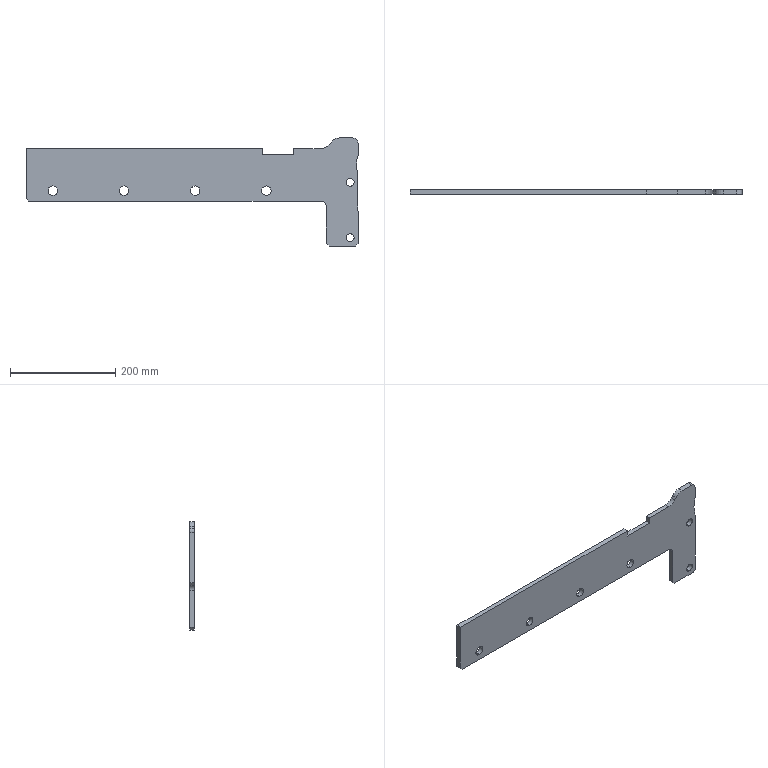Part | SolidWorks | features FlatPattern 1, SMBaseFlange 1, SheetMetal 1 | 1 solid | 36 faces | box 630 x 9 x 205 mm | volume 602554 mm3 | cylinder 18 | plane 18 | commonest cylinder face diameters 18 x8 15 x4 20 x2 40 x2 100 x2
STEP:
#1=CARTESIAN_POINT('',(615.,-9.,-176.5));
#2=VERTEX_POINT('',#1);
#3=CARTESIAN_POINT('',(615.,-9.,-161.5));
#4=VERTEX_POINT('',#3);
#5=CARTESIAN_POINT('',(615.,-9.,-169.));
#6=DIRECTION('',(0.,1.,0.));
#7=DIRECTION('',(0.,0.,1.));
#8=AXIS2_PLACEMENT_3D('',#5,#6,#7);
#9=CIRCLE('',#8,7.5);
#10=EDGE_CURVE('',#2,#4,#9,.T.);
#11=ORIENTED_EDGE('',*,*,#10,.F.);
#12=CARTESIAN_POINT('',(615.,0.,-176.5));
#13=VERTEX_POINT('',#12);
#14=CARTESIAN_POINT('',(615.,-9.,-176.5));
#15=DIRECTION('',(0.,1.,0.));
#16=VECTOR('',#15,1000.);
#17=LINE('',#14,#16);
#18=EDGE_CURVE('',#2,#13,#17,.T.);
#19=ORIENTED_EDGE('',*,*,#18,.T.);
#20=CARTESIAN_POINT('',(615.,0.,-161.5));
#21=VERTEX_POINT('',#20);
#22=CARTESIAN_POINT('',(615.,0.,-169.));
#23=DIRECTION('',(0.,1.,0.));
#24=DIRECTION('',(0.,0.,1.));
#25=AXIS2_PLACEMENT_3D('',#22,#23,#24);
#26=CIRCLE('',#25,7.5);
#27=EDGE_CURVE('',#13,#21,#26,.T.);
#28=ORIENTED_EDGE('',*,*,#27,.T.);
#29=CARTESIAN_POINT('',(615.,-9.,-161.5));
#30=DIRECTION('',(0.,1.,0.));
#31=VECTOR('',#30,1000.);
#32=LINE('',#29,#31);
#33=EDGE_CURVE('',#4,#21,#32,.T.);
#34=ORIENTED_EDGE('',*,*,#33,.F.);
#35=EDGE_LOOP('',(#11,#19,#28,#34));
#36=FACE_OUTER_BOUND('',#35,.T.);
#37=CARTESIAN_POINT('',(615.,-9.,-169.));
#38=DIRECTION('',(0.,1.,0.));
#39=DIRECTION('',(0.,0.,1.));
#40=AXIS2_PLACEMENT_3D('',#37,#38,#39);
#41=CYLINDRICAL_SURFACE('',#40,7.5);
#42=ADVANCED_FACE('',(#36),#41,.F.);
#43=CARTESIAN_POINT('',(615.,-9.,-71.5));
#44=VERTEX_POINT('',#43);
#45=CARTESIAN_POINT('',(615.,-9.,-56.5));
#46=VERTEX_POINT('',#45);
#47=CARTESIAN_POINT('',(615.,-9.,-64.));
#48=DIRECTION('',(0.,1.,0.));
#49=DIRECTION('',(0.,0.,1.));
#50=AXIS2_PLACEMENT_3D('',#47,#48,#49);
#51=CIRCLE('',#50,7.5);
#52=EDGE_CURVE('',#44,#46,#51,.T.);
#53=ORIENTED_EDGE('',*,*,#52,.F.);
#54=CARTESIAN_POINT('',(615.,0.,-71.5));
#55=VERTEX_POINT('',#54);
#56=CARTESIAN_POINT('',(615.,-9.,-71.5));
#57=DIRECTION('',(0.,1.,0.));
#58=VECTOR('',#57,1000.);
#59=LINE('',#56,#58);
#60=EDGE_CURVE('',#44,#55,#59,.T.);
#61=ORIENTED_EDGE('',*,*,#60,.T.);
#62=CARTESIAN_POINT('',(615.,0.,-56.5));
#63=VERTEX_POINT('',#62);
#64=CARTESIAN_POINT('',(615.,0.,-64.));
#65=DIRECTION('',(0.,1.,0.));
#66=DIRECTION('',(0.,0.,1.));
#67=AXIS2_PLACEMENT_3D('',#64,#65,#66);
#68=CIRCLE('',#67,7.5);
#69=EDGE_CURVE('',#55,#63,#68,.T.);
#70=ORIENTED_EDGE('',*,*,#69,.T.);
#71=CARTESIAN_POINT('',(615.,-9.,-56.5));
#72=DIRECTION('',(0.,1.,0.));
#73=VECTOR('',#72,1000.);
#74=LINE('',#71,#73);
#75=EDGE_CURVE('',#46,#63,#74,.T.);
#76=ORIENTED_EDGE('',*,*,#75,.F.);
#77=EDGE_LOOP('',(#53,#61,#70,#76));
#78=FACE_OUTER_BOUND('',#77,.T.);
#79=CARTESIAN_POINT('',(615.,-9.,-64.));
#80=DIRECTION('',(0.,1.,0.));
#81=DIRECTION('',(0.,0.,1.));
#82=AXIS2_PLACEMENT_3D('',#79,#80,#81);
#83=CYLINDRICAL_SURFACE('',#82,7.5);
#84=ADVANCED_FACE('',(#78),#83,.F.);
#85=CARTESIAN_POINT('',(456.,-9.,-89.));
#86=VERTEX_POINT('',#85);
#87=CARTESIAN_POINT('',(456.,-9.,-71.));
#88=VERTEX_POINT('',#87);
#89=CARTESIAN_POINT('',(456.,-9.,-80.));
#90=DIRECTION('',(0.,1.,0.));
#91=DIRECTION('',(0.,0.,1.));
#92=AXIS2_PLACEMENT_3D('',#89,#90,#91);
#93=CIRCLE('',#92,9.);
#94=EDGE_CURVE('',#86,#88,#93,.T.);
#95=ORIENTED_EDGE('',*,*,#94,.F.);
#96=CARTESIAN_POINT('',(456.,0.,-89.));
#97=VERTEX_POINT('',#96);
#98=CARTESIAN_POINT('',(456.,-9.,-89.));
#99=DIRECTION('',(0.,1.,0.));
#100=VECTOR('',#99,1000.);
#101=LINE('',#98,#100);
#102=EDGE_CURVE('',#86,#97,#101,.T.);
#103=ORIENTED_EDGE('',*,*,#102,.T.);
#104=CARTESIAN_POINT('',(456.,0.,-71.));
#105=VERTEX_POINT('',#104);
#106=CARTESIAN_POINT('',(456.,0.,-80.));
#107=DIRECTION('',(0.,1.,0.));
#108=DIRECTION('',(0.,0.,1.));
#109=AXIS2_PLACEMENT_3D('',#106,#107,#108);
#110=CIRCLE('',#109,9.);
#111=EDGE_CURVE('',#97,#105,#110,.T.);
#112=ORIENTED_EDGE('',*,*,#111,.T.);
#113=CARTESIAN_POINT('',(456.,-9.,-71.));
#114=DIRECTION('',(0.,1.,0.));
#115=VECTOR('',#114,1000.);
#116=LINE('',#113,#115);
#117=EDGE_CURVE('',#88,#105,#116,.T.);
#118=ORIENTED_EDGE('',*,*,#117,.F.);
#119=EDGE_LOOP('',(#95,#103,#112,#118));
#120=FACE_OUTER_BOUND('',#119,.T.);
#121=CARTESIAN_POINT('',(456.,-9.,-80.));
#122=DIRECTION('',(0.,1.,0.));
#123=DIRECTION('',(0.,0.,1.));
#124=AXIS2_PLACEMENT_3D('',#121,#122,#123);
#125=CYLINDRICAL_SURFACE('',#124,9.);
#126=ADVANCED_FACE('',(#120),#125,.F.);
#127=CARTESIAN_POINT('',(321.,-9.,-89.));
#128=VERTEX_POINT('',#127);
#129=CARTESIAN_POINT('',(321.,-9.,-71.));
#130=VERTEX_POINT('',#129);
#131=CARTESIAN_POINT('',(321.,-9.,-80.));
#132=DIRECTION('',(0.,1.,0.));
#133=DIRECTION('',(0.,0.,1.));
#134=AXIS2_PLACEMENT_3D('',#131,#132,#133);
#135=CIRCLE('',#134,9.);
#136=EDGE_CURVE('',#128,#130,#135,.T.);
#137=ORIENTED_EDGE('',*,*,#136,.F.);
#138=CARTESIAN_POINT('',(321.,0.,-89.));
#139=VERTEX_POINT('',#138);
#140=CARTESIAN_POINT('',(321.,-9.,-89.));
#141=DIRECTION('',(0.,1.,0.));
#142=VECTOR('',#141,1000.);
#143=LINE('',#140,#142);
#144=EDGE_CURVE('',#128,#139,#143,.T.);
#145=ORIENTED_EDGE('',*,*,#144,.T.);
#146=CARTESIAN_POINT('',(321.,0.,-71.));
#147=VERTEX_POINT('',#146);
#148=CARTESIAN_POINT('',(321.,0.,-80.));
#149=DIRECTION('',(0.,1.,0.));
#150=DIRECTION('',(0.,0.,1.));
#151=AXIS2_PLACEMENT_3D('',#148,#149,#150);
#152=CIRCLE('',#151,9.);
#153=EDGE_CURVE('',#139,#147,#152,.T.);
#154=ORIENTED_EDGE('',*,*,#153,.T.);
#155=CARTESIAN_POINT('',(321.,-9.,-71.));
#156=DIRECTION('',(0.,1.,0.));
#157=VECTOR('',#156,1000.);
#158=LINE('',#155,#157);
#159=EDGE_CURVE('',#130,#147,#158,.T.);
#160=ORIENTED_EDGE('',*,*,#159,.F.);
#161=EDGE_LOOP('',(#137,#145,#154,#160));
#162=FACE_OUTER_BOUND('',#161,.T.);
#163=CARTESIAN_POINT('',(321.,-9.,-80.));
#164=DIRECTION('',(0.,1.,0.));
#165=DIRECTION('',(0.,0.,1.));
#166=AXIS2_PLACEMENT_3D('',#163,#164,#165);
#167=CYLINDRICAL_SURFACE('',#166,9.);
#168=ADVANCED_FACE('',(#162),#167,.F.);
#169=CARTESIAN_POINT('',(186.,-9.,-89.));
#170=VERTEX_POINT('',#169);
#171=CARTESIAN_POINT('',(186.,-9.,-71.));
#172=VERTEX_POINT('',#171);
#173=CARTESIAN_POINT('',(186.,-9.,-80.));
#174=DIRECTION('',(0.,1.,0.));
#175=DIRECTION('',(0.,0.,1.));
#176=AXIS2_PLACEMENT_3D('',#173,#174,#175);
#177=CIRCLE('',#176,9.);
#178=EDGE_CURVE('',#170,#172,#177,.T.);
#179=ORIENTED_EDGE('',*,*,#178,.F.);
#180=CARTESIAN_POINT('',(186.,0.,-89.));
#181=VERTEX_POINT('',#180);
#182=CARTESIAN_POINT('',(186.,-9.,-89.));
#183=DIRECTION('',(0.,1.,0.));
#184=VECTOR('',#183,1000.);
#185=LINE('',#182,#184);
#186=EDGE_CURVE('',#170,#181,#185,.T.);
#187=ORIENTED_EDGE('',*,*,#186,.T.);
#188=CARTESIAN_POINT('',(186.,0.,-71.));
#189=VERTEX_POINT('',#188);
#190=CARTESIAN_POINT('',(186.,0.,-80.));
#191=DIRECTION('',(0.,1.,0.));
#192=DIRECTION('',(0.,0.,1.));
#193=AXIS2_PLACEMENT_3D('',#190,#191,#192);
#194=CIRCLE('',#193,9.);
#195=EDGE_CURVE('',#181,#189,#194,.T.);
#196=ORIENTED_EDGE('',*,*,#195,.T.);
#197=CARTESIAN_POINT('',(186.,-9.,-71.));
#198=DIRECTION('',(0.,1.,0.));
#199=VECTOR('',#198,1000.);
#200=LINE('',#197,#199);
#201=EDGE_CURVE('',#172,#189,#200,.T.);
#202=ORIENTED_EDGE('',*,*,#201,.F.);
#203=EDGE_LOOP('',(#179,#187,#196,#202));
#204=FACE_OUTER_BOUND('',#203,.T.);
#205=CARTESIAN_POINT('',(186.,-9.,-80.));
#206=DIRECTION('',(0.,1.,0.));
#207=DIRECTION('',(0.,0.,1.));
#208=AXIS2_PLACEMENT_3D('',#205,#206,#207);
#209=CYLINDRICAL_SURFACE('',#208,9.);
#210=ADVANCED_FACE('',(#204),#209,.F.);
#211=CARTESIAN_POINT('',(51.,-9.,-89.));
#212=VERTEX_POINT('',#211);
#213=CARTESIAN_POINT('',(51.,-9.,-71.));
#214=VERTEX_POINT('',#213);
#215=CARTESIAN_POINT('',(51.,-9.,-80.));
#216=DIRECTION('',(0.,1.,0.));
#217=DIRECTION('',(0.,0.,1.));
#218=AXIS2_PLACEMENT_3D('',#215,#216,#217);
#219=CIRCLE('',#218,9.);
#220=EDGE_CURVE('',#212,#214,#219,.T.);
#221=ORIENTED_EDGE('',*,*,#220,.F.);
#222=CARTESIAN_POINT('',(51.,0.,-89.));
#223=VERTEX_POINT('',#222);
#224=CARTESIAN_POINT('',(51.,-9.,-89.));
#225=DIRECTION('',(0.,1.,0.));
#226=VECTOR('',#225,1000.);
#227=LINE('',#224,#226);
#228=EDGE_CURVE('',#212,#223,#227,.T.);
#229=ORIENTED_EDGE('',*,*,#228,.T.);
#230=CARTESIAN_POINT('',(51.,0.,-71.));
#231=VERTEX_POINT('',#230);
#232=CARTESIAN_POINT('',(51.,0.,-80.));
#233=DIRECTION('',(0.,1.,0.));
#234=DIRECTION('',(0.,0.,1.));
#235=AXIS2_PLACEMENT_3D('',#232,#233,#234);
#236=CIRCLE('',#235,9.);
#237=EDGE_CURVE('',#223,#231,#236,.T.);
#238=ORIENTED_EDGE('',*,*,#237,.T.);
#239=CARTESIAN_POINT('',(51.,-9.,-71.));
#240=DIRECTION('',(0.,1.,0.));
#241=VECTOR('',#240,1000.);
#242=LINE('',#239,#241);
#243=EDGE_CURVE('',#214,#231,#242,.T.);
#244=ORIENTED_EDGE('',*,*,#243,.F.);
#245=EDGE_LOOP('',(#221,#229,#238,#244));
#246=FACE_OUTER_BOUND('',#245,.T.);
#247=CARTESIAN_POINT('',(51.,-9.,-80.));
#248=DIRECTION('',(0.,1.,0.));
#249=DIRECTION('',(0.,0.,1.));
#250=AXIS2_PLACEMENT_3D('',#247,#248,#249);
#251=CYLINDRICAL_SURFACE('',#250,9.);
#252=ADVANCED_FACE('',(#246),#251,.F.);
#253=CARTESIAN_POINT('',(0.,0.,-95.));
#254=VERTEX_POINT('',#253);
#255=CARTESIAN_POINT('',(0.,0.,0.));
#256=VERTEX_POINT('',#255);
#257=CARTESIAN_POINT('',(0.,0.,-95.));
#258=DIRECTION('',(0.,0.,1.));
#259=VECTOR('',#258,1000.);
#260=LINE('',#257,#259);
#261=EDGE_CURVE('',#254,#256,#260,.T.);
#262=ORIENTED_EDGE('',*,*,#261,.F.);
#263=CARTESIAN_POINT('',(0.,-9.,-95.));
#264=VERTEX_POINT('',#263);
#265=CARTESIAN_POINT('',(0.,-9.,-95.));
#266=DIRECTION('',(0.,1.,0.));
#267=VECTOR('',#266,1000.);
#268=LINE('',#265,#267);
#269=EDGE_CURVE('',#264,#254,#268,.T.);
#270=ORIENTED_EDGE('',*,*,#269,.F.);
#271=CARTESIAN_POINT('',(0.,-9.,0.));
#272=VERTEX_POINT('',#271);
#273=CARTESIAN_POINT('',(0.,-9.,-95.));
#274=DIRECTION('',(0.,0.,1.));
#275=VECTOR('',#274,1000.);
#276=LINE('',#273,#275);
#277=EDGE_CURVE('',#264,#272,#276,.T.);
#278=ORIENTED_EDGE('',*,*,#277,.T.);
#279=CARTESIAN_POINT('',(0.,-9.,0.));
#280=DIRECTION('',(0.,1.,0.));
#281=VECTOR('',#280,1000.);
#282=LINE('',#279,#281);
#283=EDGE_CURVE('',#272,#256,#282,.T.);
#284=ORIENTED_EDGE('',*,*,#283,.T.);
#285=EDGE_LOOP('',(#262,#270,#278,#284));
#286=FACE_OUTER_BOUND('',#285,.T.);
#287=CARTESIAN_POINT('',(0.,-9.,-95.));
#288=DIRECTION('',(-1.,0.,0.));
#289=DIRECTION('',(0.,0.,1.));
#290=AXIS2_PLACEMENT_3D('',#287,#288,#289);
#291=PLANE('',#290);
#292=ADVANCED_FACE('',(#286),#291,.T.);
#293=CARTESIAN_POINT('',(5.,0.,-100.));
#294=VERTEX_POINT('',#293);
#295=CARTESIAN_POINT('',(5.,0.,-100.));
#296=DIRECTION('',(-0.7071,0.,0.7071));
#297=VECTOR('',#296,1000.);
#298=LINE('',#295,#297);
#299=EDGE_CURVE('',#294,#254,#298,.T.);
#300=ORIENTED_EDGE('',*,*,#299,.F.);
#301=CARTESIAN_POINT('',(5.,-9.,-100.));
#302=VERTEX_POINT('',#301);
#303=CARTESIAN_POINT('',(5.,-9.,-100.));
#304=DIRECTION('',(0.,1.,0.));
#305=VECTOR('',#304,1000.);
#306=LINE('',#303,#305);
#307=EDGE_CURVE('',#302,#294,#306,.T.);
#308=ORIENTED_EDGE('',*,*,#307,.F.);
#309=CARTESIAN_POINT('',(5.,-9.,-100.));
#310=DIRECTION('',(-0.7071,0.,0.7071));
#311=VECTOR('',#310,1000.);
#312=LINE('',#309,#311);
#313=EDGE_CURVE('',#302,#264,#312,.T.);
#314=ORIENTED_EDGE('',*,*,#313,.T.);
#315=ORIENTED_EDGE('',*,*,#269,.T.);
#316=EDGE_LOOP('',(#300,#308,#314,#315));
#317=FACE_OUTER_BOUND('',#316,.T.);
#318=CARTESIAN_POINT('',(5.,-9.,-100.));
#319=DIRECTION('',(-0.7071,0.,-0.7071));
#320=DIRECTION('',(-0.7071,0.,0.7071));
#321=AXIS2_PLACEMENT_3D('',#318,#319,#320);
#322=PLANE('',#321);
#323=ADVANCED_FACE('',(#317),#322,.T.);
#324=CARTESIAN_POINT('',(560.,0.,-100.));
#325=VERTEX_POINT('',#324);
#326=CARTESIAN_POINT('',(560.,0.,-100.));
#327=DIRECTION('',(-1.,0.,0.));
#328=VECTOR('',#327,1000.);
#329=LINE('',#326,#328);
#330=EDGE_CURVE('',#325,#294,#329,.T.);
#331=ORIENTED_EDGE('',*,*,#330,.F.);
#332=CARTESIAN_POINT('',(560.,-9.,-100.));
#333=VERTEX_POINT('',#332);
#334=CARTESIAN_POINT('',(560.,-9.,-100.));
#335=DIRECTION('',(0.,1.,0.));
#336=VECTOR('',#335,1000.);
#337=LINE('',#334,#336);
#338=EDGE_CURVE('',#333,#325,#337,.T.);
#339=ORIENTED_EDGE('',*,*,#338,.F.);
#340=CARTESIAN_POINT('',(560.,-9.,-100.));
#341=DIRECTION('',(-1.,0.,0.));
#342=VECTOR('',#341,1000.);
#343=LINE('',#340,#342);
#344=EDGE_CURVE('',#333,#302,#343,.T.);
#345=ORIENTED_EDGE('',*,*,#344,.T.);
#346=ORIENTED_EDGE('',*,*,#307,.T.);
#347=EDGE_LOOP('',(#331,#339,#345,#346));
#348=FACE_OUTER_BOUND('',#347,.T.);
#349=CARTESIAN_POINT('',(560.,-9.,-100.));
#350=DIRECTION('',(0.,0.,-1.));
#351=DIRECTION('',(-1.,0.,0.));
#352=AXIS2_PLACEMENT_3D('',#349,#350,#351);
#353=PLANE('',#352);
#354=ADVANCED_FACE('',(#348),#353,.T.);
#355=CARTESIAN_POINT('',(570.,0.,-110.));
#356=VERTEX_POINT('',#355);
#357=CARTESIAN_POINT('',(560.,0.,-110.));
#358=DIRECTION('',(0.,-1.,0.));
#359=DIRECTION('',(0.,0.,-1.));
#360=AXIS2_PLACEMENT_3D('',#357,#358,#359);
#361=CIRCLE('',#360,10.);
#362=EDGE_CURVE('',#356,#325,#361,.T.);
#363=ORIENTED_EDGE('',*,*,#362,.F.);
#364=CARTESIAN_POINT('',(570.,-9.,-110.));
#365=VERTEX_POINT('',#364);
#366=CARTESIAN_POINT('',(570.,-9.,-110.));
#367=DIRECTION('',(0.,1.,0.));
#368=VECTOR('',#367,1000.);
#369=LINE('',#366,#368);
#370=EDGE_CURVE('',#365,#356,#369,.T.);
#371=ORIENTED_EDGE('',*,*,#370,.F.);
#372=CARTESIAN_POINT('',(560.,-9.,-110.));
#373=DIRECTION('',(0.,-1.,0.));
#374=DIRECTION('',(0.,0.,-1.));
#375=AXIS2_PLACEMENT_3D('',#372,#373,#374);
#376=CIRCLE('',#375,10.);
#377=EDGE_CURVE('',#365,#333,#376,.T.);
#378=ORIENTED_EDGE('',*,*,#377,.T.);
#379=ORIENTED_EDGE('',*,*,#338,.T.);
#380=EDGE_LOOP('',(#363,#371,#378,#379));
#381=FACE_OUTER_BOUND('',#380,.T.);
#382=CARTESIAN_POINT('',(560.,-9.,-110.));
#383=DIRECTION('',(0.,1.,0.));
#384=DIRECTION('',(0.,0.,1.));
#385=AXIS2_PLACEMENT_3D('',#382,#383,#384);
#386=CYLINDRICAL_SURFACE('',#385,10.);
#387=ADVANCED_FACE('',(#381),#386,.F.);
#388=CARTESIAN_POINT('',(570.,0.,-180.));
#389=VERTEX_POINT('',#388);
#390=CARTESIAN_POINT('',(570.,0.,-180.));
#391=DIRECTION('',(0.,0.,1.));
#392=VECTOR('',#391,1000.);
#393=LINE('',#390,#392);
#394=EDGE_CURVE('',#389,#356,#393,.T.);
#395=ORIENTED_EDGE('',*,*,#394,.F.);
#396=CARTESIAN_POINT('',(570.,-9.,-180.));
#397=VERTEX_POINT('',#396);
#398=CARTESIAN_POINT('',(570.,-9.,-180.));
#399=DIRECTION('',(0.,1.,0.));
#400=VECTOR('',#399,1000.);
#401=LINE('',#398,#400);
#402=EDGE_CURVE('',#397,#389,#401,.T.);
#403=ORIENTED_EDGE('',*,*,#402,.F.);
#404=CARTESIAN_POINT('',(570.,-9.,-180.));
#405=DIRECTION('',(0.,0.,1.));
#406=VECTOR('',#405,1000.);
#407=LINE('',#404,#406);
#408=EDGE_CURVE('',#397,#365,#407,.T.);
#409=ORIENTED_EDGE('',*,*,#408,.T.);
#410=ORIENTED_EDGE('',*,*,#370,.T.);
#411=EDGE_LOOP('',(#395,#403,#409,#410));
#412=FACE_OUTER_BOUND('',#411,.T.);
#413=CARTESIAN_POINT('',(570.,-9.,-180.));
#414=DIRECTION('',(-1.,0.,0.));
#415=DIRECTION('',(0.,0.,1.));
#416=AXIS2_PLACEMENT_3D('',#413,#414,#415);
#417=PLANE('',#416);
#418=ADVANCED_FACE('',(#412),#417,.T.);
#419=CARTESIAN_POINT('',(575.,0.,-185.));
#420=VERTEX_POINT('',#419);
#421=CARTESIAN_POINT('',(575.,0.,-185.));
#422=DIRECTION('',(-0.7071,0.,0.7071));
#423=VECTOR('',#422,1000.);
#424=LINE('',#421,#423);
#425=EDGE_CURVE('',#420,#389,#424,.T.);
#426=ORIENTED_EDGE('',*,*,#425,.F.);
#427=CARTESIAN_POINT('',(575.,-9.,-185.));
#428=VERTEX_POINT('',#427);
#429=CARTESIAN_POINT('',(575.,-9.,-185.));
#430=DIRECTION('',(0.,1.,0.));
#431=VECTOR('',#430,1000.);
#432=LINE('',#429,#431);
#433=EDGE_CURVE('',#428,#420,#432,.T.);
#434=ORIENTED_EDGE('',*,*,#433,.F.);
#435=CARTESIAN_POINT('',(575.,-9.,-185.));
#436=DIRECTION('',(-0.7071,0.,0.7071));
#437=VECTOR('',#436,1000.);
#438=LINE('',#435,#437);
#439=EDGE_CURVE('',#428,#397,#438,.T.);
#440=ORIENTED_EDGE('',*,*,#439,.T.);
#441=ORIENTED_EDGE('',*,*,#402,.T.);
#442=EDGE_LOOP('',(#426,#434,#440,#441));
#443=FACE_OUTER_BOUND('',#442,.T.);
#444=CARTESIAN_POINT('',(575.,-9.,-185.));
#445=DIRECTION('',(-0.7071,0.,-0.7071));
#446=DIRECTION('',(-0.7071,0.,0.7071));
#447=AXIS2_PLACEMENT_3D('',#444,#445,#446);
#448=PLANE('',#447);
#449=ADVANCED_FACE('',(#443),#448,.T.);
#450=CARTESIAN_POINT('',(625.,0.,-185.));
#451=VERTEX_POINT('',#450);
#452=CARTESIAN_POINT('',(625.,0.,-185.));
#453=DIRECTION('',(-1.,0.,0.));
#454=VECTOR('',#453,1000.);
#455=LINE('',#452,#454);
#456=EDGE_CURVE('',#451,#420,#455,.T.);
#457=ORIENTED_EDGE('',*,*,#456,.F.);
#458=CARTESIAN_POINT('',(625.,-9.,-185.));
#459=VERTEX_POINT('',#458);
#460=CARTESIAN_POINT('',(625.,-9.,-185.));
#461=DIRECTION('',(0.,1.,0.));
#462=VECTOR('',#461,1000.);
#463=LINE('',#460,#462);
#464=EDGE_CURVE('',#459,#451,#463,.T.);
#465=ORIENTED_EDGE('',*,*,#464,.F.);
#466=CARTESIAN_POINT('',(625.,-9.,-185.));
#467=DIRECTION('',(-1.,0.,0.));
#468=VECTOR('',#467,1000.);
#469=LINE('',#466,#468);
#470=EDGE_CURVE('',#459,#428,#469,.T.);
#471=ORIENTED_EDGE('',*,*,#470,.T.);
#472=ORIENTED_EDGE('',*,*,#433,.T.);
#473=EDGE_LOOP('',(#457,#465,#471,#472));
#474=FACE_OUTER_BOUND('',#473,.T.);
#475=CARTESIAN_POINT('',(625.,-9.,-185.));
#476=DIRECTION('',(0.,0.,-1.));
#477=DIRECTION('',(-1.,0.,0.));
#478=AXIS2_PLACEMENT_3D('',#475,#476,#477);
#479=PLANE('',#478);
#480=ADVANCED_FACE('',(#474),#479,.T.);
#481=CARTESIAN_POINT('',(630.,0.,-180.));
#482=VERTEX_POINT('',#481);
#483=CARTESIAN_POINT('',(630.,0.,-180.));
#484=DIRECTION('',(-0.7071,0.,-0.7071));
#485=VECTOR('',#484,1000.);
#486=LINE('',#483,#485);
#487=EDGE_CURVE('',#482,#451,#486,.T.);
#488=ORIENTED_EDGE('',*,*,#487,.F.);
#489=CARTESIAN_POINT('',(630.,-9.,-180.));
#490=VERTEX_POINT('',#489);
#491=CARTESIAN_POINT('',(630.,-9.,-180.));
#492=DIRECTION('',(0.,1.,0.));
#493=VECTOR('',#492,1000.);
#494=LINE('',#491,#493);
#495=EDGE_CURVE('',#490,#482,#494,.T.);
#496=ORIENTED_EDGE('',*,*,#495,.F.);
#497=CARTESIAN_POINT('',(630.,-9.,-180.));
#498=DIRECTION('',(-0.7071,0.,-0.7071));
#499=VECTOR('',#498,1000.);
#500=LINE('',#497,#499);
#501=EDGE_CURVE('',#490,#459,#500,.T.);
#502=ORIENTED_EDGE('',*,*,#501,.T.);
#503=ORIENTED_EDGE('',*,*,#464,.T.);
#504=EDGE_LOOP('',(#488,#496,#502,#503));
#505=FACE_OUTER_BOUND('',#504,.T.);
#506=CARTESIAN_POINT('',(630.,-9.,-180.));
#507=DIRECTION('',(0.7071,0.,-0.7071));
#508=DIRECTION('',(-0.7071,0.,-0.7071));
#509=AXIS2_PLACEMENT_3D('',#506,#507,#508);
#510=PLANE('',#509);
#511=ADVANCED_FACE('',(#505),#510,.T.);
#512=CARTESIAN_POINT('',(630.,0.,-55.369));
#513=VERTEX_POINT('',#512);
#514=CARTESIAN_POINT('',(630.,0.,-55.369));
#515=DIRECTION('',(0.,0.,-1.));
#516=VECTOR('',#515,1000.);
#517=LINE('',#514,#516);
#518=EDGE_CURVE('',#513,#482,#517,.T.);
#519=ORIENTED_EDGE('',*,*,#518,.F.);
#520=CARTESIAN_POINT('',(630.,-9.,-55.369));
#521=VERTEX_POINT('',#520);
#522=CARTESIAN_POINT('',(630.,-9.,-55.369));
#523=DIRECTION('',(0.,1.,0.));
#524=VECTOR('',#523,1000.);
#525=LINE('',#522,#524);
#526=EDGE_CURVE('',#521,#513,#525,.T.);
#527=ORIENTED_EDGE('',*,*,#526,.F.);
#528=CARTESIAN_POINT('',(630.,-9.,-55.369));
#529=DIRECTION('',(0.,0.,-1.));
#530=VECTOR('',#529,1000.);
#531=LINE('',#528,#530);
#532=EDGE_CURVE('',#521,#490,#531,.T.);
#533=ORIENTED_EDGE('',*,*,#532,.T.);
#534=ORIENTED_EDGE('',*,*,#495,.T.);
#535=EDGE_LOOP('',(#519,#527,#533,#534));
#536=FACE_OUTER_BOUND('',#535,.T.);
#537=CARTESIAN_POINT('',(630.,-9.,-55.369));
#538=DIRECTION('',(1.,0.,0.));
#539=DIRECTION('',(0.,0.,-1.));
#540=AXIS2_PLACEMENT_3D('',#537,#538,#539);
#541=PLANE('',#540);
#542=ADVANCED_FACE('',(#536),#541,.T.);
#543=CARTESIAN_POINT('',(628.5,0.,-43.214));
#544=VERTEX_POINT('',#543);
#545=CARTESIAN_POINT('',(580.,0.,-55.369));
#546=DIRECTION('',(0.,1.,0.));
#547=DIRECTION('',(0.,0.,1.));
#548=AXIS2_PLACEMENT_3D('',#545,#546,#547);
#549=CIRCLE('',#548,50.);
#550=EDGE_CURVE('',#544,#513,#549,.T.);
#551=ORIENTED_EDGE('',*,*,#550,.F.);
#552=CARTESIAN_POINT('',(628.5,-9.,-43.214));
#553=VERTEX_POINT('',#552);
#554=CARTESIAN_POINT('',(628.5,-9.,-43.214));
#555=DIRECTION('',(0.,1.,0.));
#556=VECTOR('',#555,1000.);
#557=LINE('',#554,#556);
#558=EDGE_CURVE('',#553,#544,#557,.T.);
#559=ORIENTED_EDGE('',*,*,#558,.F.);
#560=CARTESIAN_POINT('',(580.,-9.,-55.369));
#561=DIRECTION('',(0.,1.,0.));
#562=DIRECTION('',(0.,0.,1.));
#563=AXIS2_PLACEMENT_3D('',#560,#561,#562);
#564=CIRCLE('',#563,50.);
#565=EDGE_CURVE('',#553,#521,#564,.T.);
#566=ORIENTED_EDGE('',*,*,#565,.T.);
#567=ORIENTED_EDGE('',*,*,#526,.T.);
#568=EDGE_LOOP('',(#551,#559,#566,#567));
#569=FACE_OUTER_BOUND('',#568,.T.);
#570=CARTESIAN_POINT('',(580.,-9.,-55.369));
#571=DIRECTION('',(0.,1.,0.));
#572=DIRECTION('',(0.,0.,1.));
#573=AXIS2_PLACEMENT_3D('',#570,#571,#572);
#574=CYLINDRICAL_SURFACE('',#573,50.);
#575=ADVANCED_FACE('',(#569),#574,.T.);
#576=CARTESIAN_POINT('',(630.,0.,-14.));
#577=VERTEX_POINT('',#576);
#578=CARTESIAN_POINT('',(677.,0.,-31.059));
#579=DIRECTION('',(0.,-1.,0.));
#580=DIRECTION('',(0.,0.,1.));
#581=AXIS2_PLACEMENT_3D('',#578,#579,#580);
#582=CIRCLE('',#581,50.);
#583=EDGE_CURVE('',#577,#544,#582,.T.);
#584=ORIENTED_EDGE('',*,*,#583,.F.);
#585=CARTESIAN_POINT('',(630.,-9.,-14.));
#586=VERTEX_POINT('',#585);
#587=CARTESIAN_POINT('',(630.,-9.,-14.));
#588=DIRECTION('',(0.,1.,0.));
#589=VECTOR('',#588,1000.);
#590=LINE('',#587,#589);
#591=EDGE_CURVE('',#586,#577,#590,.T.);
#592=ORIENTED_EDGE('',*,*,#591,.F.);
#593=CARTESIAN_POINT('',(677.,-9.,-31.059));
#594=DIRECTION('',(0.,-1.,0.));
#595=DIRECTION('',(0.,0.,1.));
#596=AXIS2_PLACEMENT_3D('',#593,#594,#595);
#597=CIRCLE('',#596,50.);
#598=EDGE_CURVE('',#586,#553,#597,.T.);
#599=ORIENTED_EDGE('',*,*,#598,.T.);
#600=ORIENTED_EDGE('',*,*,#558,.T.);
#601=EDGE_LOOP('',(#584,#592,#599,#600));
#602=FACE_OUTER_BOUND('',#601,.T.);
#603=CARTESIAN_POINT('',(677.,-9.,-31.059));
#604=DIRECTION('',(0.,1.,0.));
#605=DIRECTION('',(0.,0.,1.));
#606=AXIS2_PLACEMENT_3D('',#603,#604,#605);
#607=CYLINDRICAL_SURFACE('',#606,50.);
#608=ADVANCED_FACE('',(#602),#607,.F.);
#609=CARTESIAN_POINT('',(630.,0.,10.));
#610=VERTEX_POINT('',#609);
#611=CARTESIAN_POINT('',(630.,0.,10.));
#612=DIRECTION('',(0.,0.,-1.));
#613=VECTOR('',#612,1000.);
#614=LINE('',#611,#613);
#615=EDGE_CURVE('',#610,#577,#614,.T.);
#616=ORIENTED_EDGE('',*,*,#615,.F.);
#617=CARTESIAN_POINT('',(630.,-9.,10.));
#618=VERTEX_POINT('',#617);
#619=CARTESIAN_POINT('',(630.,-9.,10.));
#620=DIRECTION('',(0.,1.,0.));
#621=VECTOR('',#620,1000.);
#622=LINE('',#619,#621);
#623=EDGE_CURVE('',#618,#610,#622,.T.);
#624=ORIENTED_EDGE('',*,*,#623,.F.);
#625=CARTESIAN_POINT('',(630.,-9.,10.));
#626=DIRECTION('',(0.,0.,-1.));
#627=VECTOR('',#626,1000.);
#628=LINE('',#625,#627);
#629=EDGE_CURVE('',#618,#586,#628,.T.);
#630=ORIENTED_EDGE('',*,*,#629,.T.);
#631=ORIENTED_EDGE('',*,*,#591,.T.);
#632=EDGE_LOOP('',(#616,#624,#630,#631));
#633=FACE_OUTER_BOUND('',#632,.T.);
#634=CARTESIAN_POINT('',(630.,-9.,10.));
#635=DIRECTION('',(1.,0.,0.));
#636=DIRECTION('',(0.,0.,-1.));
#637=AXIS2_PLACEMENT_3D('',#634,#635,#636);
#638=PLANE('',#637);
#639=ADVANCED_FACE('',(#633),#638,.T.);
#640=CARTESIAN_POINT('',(620.,0.,20.));
#641=VERTEX_POINT('',#640);
#642=CARTESIAN_POINT('',(620.,0.,10.));
#643=DIRECTION('',(0.,1.,0.));
#644=DIRECTION('',(0.,0.,1.));
#645=AXIS2_PLACEMENT_3D('',#642,#643,#644);
#646=CIRCLE('',#645,10.);
#647=EDGE_CURVE('',#641,#610,#646,.T.);
#648=ORIENTED_EDGE('',*,*,#647,.F.);
#649=CARTESIAN_POINT('',(620.,-9.,20.));
#650=VERTEX_POINT('',#649);
#651=CARTESIAN_POINT('',(620.,-9.,20.));
#652=DIRECTION('',(0.,1.,0.));
#653=VECTOR('',#652,1000.);
#654=LINE('',#651,#653);
#655=EDGE_CURVE('',#650,#641,#654,.T.);
#656=ORIENTED_EDGE('',*,*,#655,.F.);
#657=CARTESIAN_POINT('',(620.,-9.,10.));
#658=DIRECTION('',(0.,1.,0.));
#659=DIRECTION('',(0.,0.,1.));
#660=AXIS2_PLACEMENT_3D('',#657,#658,#659);
#661=CIRCLE('',#660,10.);
#662=EDGE_CURVE('',#650,#618,#661,.T.);
#663=ORIENTED_EDGE('',*,*,#662,.T.);
#664=ORIENTED_EDGE('',*,*,#623,.T.);
#665=EDGE_LOOP('',(#648,#656,#663,#664));
#666=FACE_OUTER_BOUND('',#665,.T.);
#667=CARTESIAN_POINT('',(620.,-9.,10.));
#668=DIRECTION('',(0.,1.,0.));
#669=DIRECTION('',(0.,0.,1.));
#670=AXIS2_PLACEMENT_3D('',#667,#668,#669);
#671=CYLINDRICAL_SURFACE('',#670,10.);
#672=ADVANCED_FACE('',(#666),#671,.T.);
#673=CARTESIAN_POINT('',(595.,0.,20.));
#674=VERTEX_POINT('',#673);
#675=CARTESIAN_POINT('',(595.,0.,20.));
#676=DIRECTION('',(1.,0.,0.));
#677=VECTOR('',#676,1000.);
#678=LINE('',#675,#677);
#679=EDGE_CURVE('',#674,#641,#678,.T.);
#680=ORIENTED_EDGE('',*,*,#679,.F.);
#681=CARTESIAN_POINT('',(595.,-9.,20.));
#682=VERTEX_POINT('',#681);
#683=CARTESIAN_POINT('',(595.,-9.,20.));
#684=DIRECTION('',(0.,1.,0.));
#685=VECTOR('',#684,1000.);
#686=LINE('',#683,#685);
#687=EDGE_CURVE('',#682,#674,#686,.T.);
#688=ORIENTED_EDGE('',*,*,#687,.F.);
#689=CARTESIAN_POINT('',(595.,-9.,20.));
#690=DIRECTION('',(1.,0.,0.));
#691=VECTOR('',#690,1000.);
#692=LINE('',#689,#691);
#693=EDGE_CURVE('',#682,#650,#692,.T.);
#694=ORIENTED_EDGE('',*,*,#693,.T.);
#695=ORIENTED_EDGE('',*,*,#655,.T.);
#696=EDGE_LOOP('',(#680,#688,#694,#695));
#697=FACE_OUTER_BOUND('',#696,.T.);
#698=CARTESIAN_POINT('',(595.,-9.,20.));
#699=DIRECTION('',(0.,0.,1.));
#700=DIRECTION('',(1.,0.,0.));
#701=AXIS2_PLACEMENT_3D('',#698,#699,#700);
#702=PLANE('',#701);
#703=ADVANCED_FACE('',(#697),#702,.T.);
#704=CARTESIAN_POINT('',(579.,0.,12.));
#705=VERTEX_POINT('',#704);
#706=CARTESIAN_POINT('',(595.,0.,0.));
#707=DIRECTION('',(0.,1.,0.));
#708=DIRECTION('',(0.,0.,1.));
#709=AXIS2_PLACEMENT_3D('',#706,#707,#708);
#710=CIRCLE('',#709,20.);
#711=EDGE_CURVE('',#705,#674,#710,.T.);
#712=ORIENTED_EDGE('',*,*,#711,.F.);
#713=CARTESIAN_POINT('',(579.,-9.,12.));
#714=VERTEX_POINT('',#713);
#715=CARTESIAN_POINT('',(579.,-9.,12.));
#716=DIRECTION('',(0.,1.,0.));
#717=VECTOR('',#716,1000.);
#718=LINE('',#715,#717);
#719=EDGE_CURVE('',#714,#705,#718,.T.);
#720=ORIENTED_EDGE('',*,*,#719,.F.);
#721=CARTESIAN_POINT('',(595.,-9.,0.));
#722=DIRECTION('',(0.,1.,0.));
#723=DIRECTION('',(0.,0.,1.));
#724=AXIS2_PLACEMENT_3D('',#721,#722,#723);
#725=CIRCLE('',#724,20.);
#726=EDGE_CURVE('',#714,#682,#725,.T.);
#727=ORIENTED_EDGE('',*,*,#726,.T.);
#728=ORIENTED_EDGE('',*,*,#687,.T.);
#729=EDGE_LOOP('',(#712,#720,#727,#728));
#730=FACE_OUTER_BOUND('',#729,.T.);
#731=CARTESIAN_POINT('',(595.,-9.,0.));
#732=DIRECTION('',(0.,1.,0.));
#733=DIRECTION('',(0.,0.,1.));
#734=AXIS2_PLACEMENT_3D('',#731,#732,#733);
#735=CYLINDRICAL_SURFACE('',#734,20.);
#736=ADVANCED_FACE('',(#730),#735,.T.);
#737=CARTESIAN_POINT('',(576.,0.,8.));
#738=VERTEX_POINT('',#737);
#739=CARTESIAN_POINT('',(576.,0.,8.));
#740=DIRECTION('',(0.6,0.,0.8));
#741=VECTOR('',#740,1000.);
#742=LINE('',#739,#741);
#743=EDGE_CURVE('',#738,#705,#742,.T.);
#744=ORIENTED_EDGE('',*,*,#743,.F.);
#745=CARTESIAN_POINT('',(576.,-9.,8.));
#746=VERTEX_POINT('',#745);
#747=CARTESIAN_POINT('',(576.,-9.,8.));
#748=DIRECTION('',(0.,1.,0.));
#749=VECTOR('',#748,1000.);
#750=LINE('',#747,#749);
#751=EDGE_CURVE('',#746,#738,#750,.T.);
#752=ORIENTED_EDGE('',*,*,#751,.F.);
#753=CARTESIAN_POINT('',(576.,-9.,8.));
#754=DIRECTION('',(0.6,0.,0.8));
#755=VECTOR('',#754,1000.);
#756=LINE('',#753,#755);
#757=EDGE_CURVE('',#746,#714,#756,.T.);
#758=ORIENTED_EDGE('',*,*,#757,.T.);
#759=ORIENTED_EDGE('',*,*,#719,.T.);
#760=EDGE_LOOP('',(#744,#752,#758,#759));
#761=FACE_OUTER_BOUND('',#760,.T.);
#762=CARTESIAN_POINT('',(576.,-9.,8.));
#763=DIRECTION('',(-0.8,0.,0.6));
#764=DIRECTION('',(0.6,0.,0.8));
#765=AXIS2_PLACEMENT_3D('',#762,#763,#764);
#766=PLANE('',#765);
#767=ADVANCED_FACE('',(#761),#766,.T.);
#768=CARTESIAN_POINT('',(560.,0.,0.));
#769=VERTEX_POINT('',#768);
#770=CARTESIAN_POINT('',(560.,0.,20.));
#771=DIRECTION('',(0.,-1.,0.));
#772=DIRECTION('',(0.,0.,-1.));
#773=AXIS2_PLACEMENT_3D('',#770,#771,#772);
#774=CIRCLE('',#773,20.);
#775=EDGE_CURVE('',#769,#738,#774,.T.);
#776=ORIENTED_EDGE('',*,*,#775,.F.);
#777=CARTESIAN_POINT('',(560.,-9.,0.));
#778=VERTEX_POINT('',#777);
#779=CARTESIAN_POINT('',(560.,-9.,0.));
#780=DIRECTION('',(0.,1.,0.));
#781=VECTOR('',#780,1000.);
#782=LINE('',#779,#781);
#783=EDGE_CURVE('',#778,#769,#782,.T.);
#784=ORIENTED_EDGE('',*,*,#783,.F.);
#785=CARTESIAN_POINT('',(560.,-9.,20.));
#786=DIRECTION('',(0.,-1.,0.));
#787=DIRECTION('',(0.,0.,-1.));
#788=AXIS2_PLACEMENT_3D('',#785,#786,#787);
#789=CIRCLE('',#788,20.);
#790=EDGE_CURVE('',#778,#746,#789,.T.);
#791=ORIENTED_EDGE('',*,*,#790,.T.);
#792=ORIENTED_EDGE('',*,*,#751,.T.);
#793=EDGE_LOOP('',(#776,#784,#791,#792));
#794=FACE_OUTER_BOUND('',#793,.T.);
#795=CARTESIAN_POINT('',(560.,-9.,20.));
#796=DIRECTION('',(0.,1.,0.));
#797=DIRECTION('',(0.,0.,1.));
#798=AXIS2_PLACEMENT_3D('',#795,#796,#797);
#799=CYLINDRICAL_SURFACE('',#798,20.);
#800=ADVANCED_FACE('',(#794),#799,.F.);
#801=CARTESIAN_POINT('',(508.,0.,0.));
#802=VERTEX_POINT('',#801);
#803=CARTESIAN_POINT('',(508.,0.,0.));
#804=DIRECTION('',(1.,0.,0.));
#805=VECTOR('',#804,1000.);
#806=LINE('',#803,#805);
#807=EDGE_CURVE('',#802,#769,#806,.T.);
#808=ORIENTED_EDGE('',*,*,#807,.F.);
#809=CARTESIAN_POINT('',(508.,-9.,0.));
#810=VERTEX_POINT('',#809);
#811=CARTESIAN_POINT('',(508.,-9.,0.));
#812=DIRECTION('',(0.,1.,0.));
#813=VECTOR('',#812,1000.);
#814=LINE('',#811,#813);
#815=EDGE_CURVE('',#810,#802,#814,.T.);
#816=ORIENTED_EDGE('',*,*,#815,.F.);
#817=CARTESIAN_POINT('',(508.,-9.,0.));
#818=DIRECTION('',(1.,0.,0.));
#819=VECTOR('',#818,1000.);
#820=LINE('',#817,#819);
#821=EDGE_CURVE('',#810,#778,#820,.T.);
#822=ORIENTED_EDGE('',*,*,#821,.T.);
#823=ORIENTED_EDGE('',*,*,#783,.T.);
#824=EDGE_LOOP('',(#808,#816,#822,#823));
#825=FACE_OUTER_BOUND('',#824,.T.);
#826=CARTESIAN_POINT('',(508.,-9.,0.));
#827=DIRECTION('',(0.,0.,1.));
#828=DIRECTION('',(1.,0.,0.));
#829=AXIS2_PLACEMENT_3D('',#826,#827,#828);
#830=PLANE('',#829);
#831=ADVANCED_FACE('',(#825),#830,.T.);
#832=CARTESIAN_POINT('',(508.,0.,-12.));
#833=VERTEX_POINT('',#832);
#834=CARTESIAN_POINT('',(508.,0.,-12.));
#835=DIRECTION('',(0.,0.,1.));
#836=VECTOR('',#835,1000.);
#837=LINE('',#834,#836);
#838=EDGE_CURVE('',#833,#802,#837,.T.);
#839=ORIENTED_EDGE('',*,*,#838,.F.);
#840=CARTESIAN_POINT('',(508.,-9.,-12.));
#841=VERTEX_POINT('',#840);
#842=CARTESIAN_POINT('',(508.,-9.,-12.));
#843=DIRECTION('',(0.,1.,0.));
#844=VECTOR('',#843,1000.);
#845=LINE('',#842,#844);
#846=EDGE_CURVE('',#841,#833,#845,.T.);
#847=ORIENTED_EDGE('',*,*,#846,.F.);
#848=CARTESIAN_POINT('',(508.,-9.,-12.));
#849=DIRECTION('',(0.,0.,1.));
#850=VECTOR('',#849,1000.);
#851=LINE('',#848,#850);
#852=EDGE_CURVE('',#841,#810,#851,.T.);
#853=ORIENTED_EDGE('',*,*,#852,.T.);
#854=ORIENTED_EDGE('',*,*,#815,.T.);
#855=EDGE_LOOP('',(#839,#847,#853,#854));
#856=FACE_OUTER_BOUND('',#855,.T.);
#857=CARTESIAN_POINT('',(508.,-9.,-12.));
#858=DIRECTION('',(-1.,0.,0.));
#859=DIRECTION('',(0.,0.,1.));
#860=AXIS2_PLACEMENT_3D('',#857,#858,#859);
#861=PLANE('',#860);
#862=ADVANCED_FACE('',(#856),#861,.T.);
#863=CARTESIAN_POINT('',(448.,0.,-12.));
#864=VERTEX_POINT('',#863);
#865=CARTESIAN_POINT('',(448.,0.,-12.));
#866=DIRECTION('',(1.,0.,0.));
#867=VECTOR('',#866,1000.);
#868=LINE('',#865,#867);
#869=EDGE_CURVE('',#864,#833,#868,.T.);
#870=ORIENTED_EDGE('',*,*,#869,.F.);
#871=CARTESIAN_POINT('',(448.,-9.,-12.));
#872=VERTEX_POINT('',#871);
#873=CARTESIAN_POINT('',(448.,-9.,-12.));
#874=DIRECTION('',(0.,1.,0.));
#875=VECTOR('',#874,1000.);
#876=LINE('',#873,#875);
#877=EDGE_CURVE('',#872,#864,#876,.T.);
#878=ORIENTED_EDGE('',*,*,#877,.F.);
#879=CARTESIAN_POINT('',(448.,-9.,-12.));
#880=DIRECTION('',(1.,0.,0.));
#881=VECTOR('',#880,1000.);
#882=LINE('',#879,#881);
#883=EDGE_CURVE('',#872,#841,#882,.T.);
#884=ORIENTED_EDGE('',*,*,#883,.T.);
#885=ORIENTED_EDGE('',*,*,#846,.T.);
#886=EDGE_LOOP('',(#870,#878,#884,#885));
#887=FACE_OUTER_BOUND('',#886,.T.);
#888=CARTESIAN_POINT('',(448.,-9.,-12.));
#889=DIRECTION('',(0.,0.,1.));
#890=DIRECTION('',(1.,0.,0.));
#891=AXIS2_PLACEMENT_3D('',#888,#889,#890);
#892=PLANE('',#891);
#893=ADVANCED_FACE('',(#887),#892,.T.);
#894=CARTESIAN_POINT('',(448.,0.,0.));
#895=VERTEX_POINT('',#894);
#896=CARTESIAN_POINT('',(448.,0.,0.));
#897=DIRECTION('',(0.,0.,-1.));
#898=VECTOR('',#897,1000.);
#899=LINE('',#896,#898);
#900=EDGE_CURVE('',#895,#864,#899,.T.);
#901=ORIENTED_EDGE('',*,*,#900,.F.);
#902=CARTESIAN_POINT('',(448.,-9.,0.));
#903=VERTEX_POINT('',#902);
#904=CARTESIAN_POINT('',(448.,-9.,0.));
#905=DIRECTION('',(0.,1.,0.));
#906=VECTOR('',#905,1000.);
#907=LINE('',#904,#906);
#908=EDGE_CURVE('',#903,#895,#907,.T.);
#909=ORIENTED_EDGE('',*,*,#908,.F.);
#910=CARTESIAN_POINT('',(448.,-9.,0.));
#911=DIRECTION('',(0.,0.,-1.));
#912=VECTOR('',#911,1000.);
#913=LINE('',#910,#912);
#914=EDGE_CURVE('',#903,#872,#913,.T.);
#915=ORIENTED_EDGE('',*,*,#914,.T.);
#916=ORIENTED_EDGE('',*,*,#877,.T.);
#917=EDGE_LOOP('',(#901,#909,#915,#916));
#918=FACE_OUTER_BOUND('',#917,.T.);
#919=CARTESIAN_POINT('',(448.,-9.,0.));
#920=DIRECTION('',(1.,0.,0.));
#921=DIRECTION('',(0.,0.,-1.));
#922=AXIS2_PLACEMENT_3D('',#919,#920,#921);
#923=PLANE('',#922);
#924=ADVANCED_FACE('',(#918),#923,.T.);
#925=CARTESIAN_POINT('',(0.,0.,0.));
#926=DIRECTION('',(1.,0.,0.));
#927=VECTOR('',#926,1000.);
#928=LINE('',#925,#927);
#929=EDGE_CURVE('',#256,#895,#928,.T.);
#930=ORIENTED_EDGE('',*,*,#929,.F.);
#931=ORIENTED_EDGE('',*,*,#283,.F.);
#932=CARTESIAN_POINT('',(0.,-9.,0.));
#933=DIRECTION('',(1.,0.,0.));
#934=VECTOR('',#933,1000.);
#935=LINE('',#932,#934);
#936=EDGE_CURVE('',#272,#903,#935,.T.);
#937=ORIENTED_EDGE('',*,*,#936,.T.);
#938=ORIENTED_EDGE('',*,*,#908,.T.);
#939=EDGE_LOOP('',(#930,#931,#937,#938));
#940=FACE_OUTER_BOUND('',#939,.T.);
#941=CARTESIAN_POINT('',(0.,-9.,0.));
#942=DIRECTION('',(0.,0.,1.));
#943=DIRECTION('',(1.,0.,0.));
#944=AXIS2_PLACEMENT_3D('',#941,#942,#943);
#945=PLANE('',#944);
#946=ADVANCED_FACE('',(#940),#945,.T.);
#947=CARTESIAN_POINT('',(615.,-9.,-169.));
#948=DIRECTION('',(0.,1.,0.));
#949=DIRECTION('',(0.,0.,1.));
#950=AXIS2_PLACEMENT_3D('',#947,#948,#949);
#951=CIRCLE('',#950,7.5);
#952=EDGE_CURVE('',#4,#2,#951,.T.);
#953=ORIENTED_EDGE('',*,*,#952,.T.);
#954=ORIENTED_EDGE('',*,*,#10,.T.);
#955=EDGE_LOOP('',(#953,#954));
#956=FACE_BOUND('',#955,.T.);
#957=CARTESIAN_POINT('',(615.,-9.,-64.));
#958=DIRECTION('',(0.,1.,0.));
#959=DIRECTION('',(0.,0.,1.));
#960=AXIS2_PLACEMENT_3D('',#957,#958,#959);
#961=CIRCLE('',#960,7.5);
#962=EDGE_CURVE('',#46,#44,#961,.T.);
#963=ORIENTED_EDGE('',*,*,#962,.T.);
#964=ORIENTED_EDGE('',*,*,#52,.T.);
#965=EDGE_LOOP('',(#963,#964));
#966=FACE_BOUND('',#965,.T.);
#967=CARTESIAN_POINT('',(456.,-9.,-80.));
#968=DIRECTION('',(0.,1.,0.));
#969=DIRECTION('',(0.,0.,1.));
#970=AXIS2_PLACEMENT_3D('',#967,#968,#969);
#971=CIRCLE('',#970,9.);
#972=EDGE_CURVE('',#88,#86,#971,.T.);
#973=ORIENTED_EDGE('',*,*,#972,.T.);
#974=ORIENTED_EDGE('',*,*,#94,.T.);
#975=EDGE_LOOP('',(#973,#974));
#976=FACE_BOUND('',#975,.T.);
#977=CARTESIAN_POINT('',(321.,-9.,-80.));
#978=DIRECTION('',(0.,1.,0.));
#979=DIRECTION('',(0.,0.,1.));
#980=AXIS2_PLACEMENT_3D('',#977,#978,#979);
#981=CIRCLE('',#980,9.);
#982=EDGE_CURVE('',#130,#128,#981,.T.);
#983=ORIENTED_EDGE('',*,*,#982,.T.);
#984=ORIENTED_EDGE('',*,*,#136,.T.);
#985=EDGE_LOOP('',(#983,#984));
#986=FACE_BOUND('',#985,.T.);
#987=CARTESIAN_POINT('',(186.,-9.,-80.));
#988=DIRECTION('',(0.,1.,0.));
#989=DIRECTION('',(0.,0.,1.));
#990=AXIS2_PLACEMENT_3D('',#987,#988,#989);
#991=CIRCLE('',#990,9.);
#992=EDGE_CURVE('',#172,#170,#991,.T.);
#993=ORIENTED_EDGE('',*,*,#992,.T.);
#994=ORIENTED_EDGE('',*,*,#178,.T.);
#995=EDGE_LOOP('',(#993,#994));
#996=FACE_BOUND('',#995,.T.);
#997=CARTESIAN_POINT('',(51.,-9.,-80.));
#998=DIRECTION('',(0.,1.,0.));
#999=DIRECTION('',(0.,0.,1.));
#1000=AXIS2_PLACEMENT_3D('',#997,#998,#999);
#1001=CIRCLE('',#1000,9.);
#1002=EDGE_CURVE('',#214,#212,#1001,.T.);
#1003=ORIENTED_EDGE('',*,*,#1002,.T.);
#1004=ORIENTED_EDGE('',*,*,#220,.T.);
#1005=EDGE_LOOP('',(#1003,#1004));
#1006=FACE_BOUND('',#1005,.T.);
#1007=ORIENTED_EDGE('',*,*,#277,.F.);
#1008=ORIENTED_EDGE('',*,*,#313,.F.);
#1009=ORIENTED_EDGE('',*,*,#344,.F.);
#1010=ORIENTED_EDGE('',*,*,#377,.F.);
#1011=ORIENTED_EDGE('',*,*,#408,.F.);
#1012=ORIENTED_EDGE('',*,*,#439,.F.);
#1013=ORIENTED_EDGE('',*,*,#470,.F.);
#1014=ORIENTED_EDGE('',*,*,#501,.F.);
#1015=ORIENTED_EDGE('',*,*,#532,.F.);
#1016=ORIENTED_EDGE('',*,*,#565,.F.);
#1017=ORIENTED_EDGE('',*,*,#598,.F.);
#1018=ORIENTED_EDGE('',*,*,#629,.F.);
#1019=ORIENTED_EDGE('',*,*,#662,.F.);
#1020=ORIENTED_EDGE('',*,*,#693,.F.);
#1021=ORIENTED_EDGE('',*,*,#726,.F.);
#1022=ORIENTED_EDGE('',*,*,#757,.F.);
#1023=ORIENTED_EDGE('',*,*,#790,.F.);
#1024=ORIENTED_EDGE('',*,*,#821,.F.);
#1025=ORIENTED_EDGE('',*,*,#852,.F.);
#1026=ORIENTED_EDGE('',*,*,#883,.F.);
#1027=ORIENTED_EDGE('',*,*,#914,.F.);
#1028=ORIENTED_EDGE('',*,*,#936,.F.);
#1029=EDGE_LOOP('',(#1007,#1008,#1009,#1010,#1011,#1012,#1013,#1014,#1015,#1016,#1017,#1018,#1019,#1020,#1021,#1022,#1023,#1024,#1025,#1026,#1027,#1028));
#1030=FACE_OUTER_BOUND('',#1029,.T.);
#1031=CARTESIAN_POINT('',(560.,-9.,20.));
#1032=DIRECTION('',(0.,-1.,0.));
#1033=DIRECTION('',(0.,0.,-1.));
#1034=AXIS2_PLACEMENT_3D('',#1031,#1032,#1033);
#1035=PLANE('',#1034);
#1036=ADVANCED_FACE('',(#956,#966,#976,#986,#996,#1006,#1030),#1035,.T.);
#1037=CARTESIAN_POINT('',(615.,0.,-169.));
#1038=DIRECTION('',(0.,1.,0.));
#1039=DIRECTION('',(0.,0.,1.));
#1040=AXIS2_PLACEMENT_3D('',#1037,#1038,#1039);
#1041=CIRCLE('',#1040,7.5);
#1042=EDGE_CURVE('',#21,#13,#1041,.T.);
#1043=ORIENTED_EDGE('',*,*,#1042,.F.);
#1044=ORIENTED_EDGE('',*,*,#27,.F.);
#1045=EDGE_LOOP('',(#1043,#1044));
#1046=FACE_BOUND('',#1045,.T.);
#1047=CARTESIAN_POINT('',(615.,0.,-64.));
#1048=DIRECTION('',(0.,1.,0.));
#1049=DIRECTION('',(0.,0.,1.));
#1050=AXIS2_PLACEMENT_3D('',#1047,#1048,#1049);
#1051=CIRCLE('',#1050,7.5);
#1052=EDGE_CURVE('',#63,#55,#1051,.T.);
#1053=ORIENTED_EDGE('',*,*,#1052,.F.);
#1054=ORIENTED_EDGE('',*,*,#69,.F.);
#1055=EDGE_LOOP('',(#1053,#1054));
#1056=FACE_BOUND('',#1055,.T.);
#1057=CARTESIAN_POINT('',(456.,0.,-80.));
#1058=DIRECTION('',(0.,1.,0.));
#1059=DIRECTION('',(0.,0.,1.));
#1060=AXIS2_PLACEMENT_3D('',#1057,#1058,#1059);
#1061=CIRCLE('',#1060,9.);
#1062=EDGE_CURVE('',#105,#97,#1061,.T.);
#1063=ORIENTED_EDGE('',*,*,#1062,.F.);
#1064=ORIENTED_EDGE('',*,*,#111,.F.);
#1065=EDGE_LOOP('',(#1063,#1064));
#1066=FACE_BOUND('',#1065,.T.);
#1067=CARTESIAN_POINT('',(321.,0.,-80.));
#1068=DIRECTION('',(0.,1.,0.));
#1069=DIRECTION('',(0.,0.,1.));
#1070=AXIS2_PLACEMENT_3D('',#1067,#1068,#1069);
#1071=CIRCLE('',#1070,9.);
#1072=EDGE_CURVE('',#147,#139,#1071,.T.);
#1073=ORIENTED_EDGE('',*,*,#1072,.F.);
#1074=ORIENTED_EDGE('',*,*,#153,.F.);
#1075=EDGE_LOOP('',(#1073,#1074));
#1076=FACE_BOUND('',#1075,.T.);
#1077=CARTESIAN_POINT('',(186.,0.,-80.));
#1078=DIRECTION('',(0.,1.,0.));
#1079=DIRECTION('',(0.,0.,1.));
#1080=AXIS2_PLACEMENT_3D('',#1077,#1078,#1079);
#1081=CIRCLE('',#1080,9.);
#1082=EDGE_CURVE('',#189,#181,#1081,.T.);
#1083=ORIENTED_EDGE('',*,*,#1082,.F.);
#1084=ORIENTED_EDGE('',*,*,#195,.F.);
#1085=EDGE_LOOP('',(#1083,#1084));
#1086=FACE_BOUND('',#1085,.T.);
#1087=CARTESIAN_POINT('',(51.,0.,-80.));
#1088=DIRECTION('',(0.,1.,0.));
#1089=DIRECTION('',(0.,0.,1.));
#1090=AXIS2_PLACEMENT_3D('',#1087,#1088,#1089);
#1091=CIRCLE('',#1090,9.);
#1092=EDGE_CURVE('',#231,#223,#1091,.T.);
#1093=ORIENTED_EDGE('',*,*,#1092,.F.);
#1094=ORIENTED_EDGE('',*,*,#237,.F.);
#1095=EDGE_LOOP('',(#1093,#1094));
#1096=FACE_BOUND('',#1095,.T.);
#1097=ORIENTED_EDGE('',*,*,#261,.T.);
#1098=ORIENTED_EDGE('',*,*,#929,.T.);
#1099=ORIENTED_EDGE('',*,*,#900,.T.);
#1100=ORIENTED_EDGE('',*,*,#869,.T.);
#1101=ORIENTED_EDGE('',*,*,#838,.T.);
#1102=ORIENTED_EDGE('',*,*,#807,.T.);
#1103=ORIENTED_EDGE('',*,*,#775,.T.);
#1104=ORIENTED_EDGE('',*,*,#743,.T.);
#1105=ORIENTED_EDGE('',*,*,#711,.T.);
#1106=ORIENTED_EDGE('',*,*,#679,.T.);
#1107=ORIENTED_EDGE('',*,*,#647,.T.);
#1108=ORIENTED_EDGE('',*,*,#615,.T.);
#1109=ORIENTED_EDGE('',*,*,#583,.T.);
#1110=ORIENTED_EDGE('',*,*,#550,.T.);
#1111=ORIENTED_EDGE('',*,*,#518,.T.);
#1112=ORIENTED_EDGE('',*,*,#487,.T.);
#1113=ORIENTED_EDGE('',*,*,#456,.T.);
#1114=ORIENTED_EDGE('',*,*,#425,.T.);
#1115=ORIENTED_EDGE('',*,*,#394,.T.);
#1116=ORIENTED_EDGE('',*,*,#362,.T.);
#1117=ORIENTED_EDGE('',*,*,#330,.T.);
#1118=ORIENTED_EDGE('',*,*,#299,.T.);
#1119=EDGE_LOOP('',(#1097,#1098,#1099,#1100,#1101,#1102,#1103,#1104,#1105,#1106,#1107,#1108,#1109,#1110,#1111,#1112,#1113,#1114,#1115,#1116,#1117,#1118));
#1120=FACE_OUTER_BOUND('',#1119,.T.);
#1121=CARTESIAN_POINT('',(560.,0.,20.));
#1122=DIRECTION('',(0.,-1.,0.));
#1123=DIRECTION('',(0.,0.,-1.));
#1124=AXIS2_PLACEMENT_3D('',#1121,#1122,#1123);
#1125=PLANE('',#1124);
#1126=ADVANCED_FACE('',(#1046,#1056,#1066,#1076,#1086,#1096,#1120),#1125,.F.);
#1127=ORIENTED_EDGE('',*,*,#228,.F.);
#1128=ORIENTED_EDGE('',*,*,#1002,.F.);
#1129=ORIENTED_EDGE('',*,*,#243,.T.);
#1130=ORIENTED_EDGE('',*,*,#1092,.T.);
#1131=EDGE_LOOP('',(#1127,#1128,#1129,#1130));
#1132=FACE_OUTER_BOUND('',#1131,.T.);
#1133=CARTESIAN_POINT('',(51.,-9.,-80.));
#1134=DIRECTION('',(0.,1.,0.));
#1135=DIRECTION('',(0.,0.,1.));
#1136=AXIS2_PLACEMENT_3D('',#1133,#1134,#1135);
#1137=CYLINDRICAL_SURFACE('',#1136,9.);
#1138=ADVANCED_FACE('',(#1132),#1137,.F.);
#1139=ORIENTED_EDGE('',*,*,#186,.F.);
#1140=ORIENTED_EDGE('',*,*,#992,.F.);
#1141=ORIENTED_EDGE('',*,*,#201,.T.);
#1142=ORIENTED_EDGE('',*,*,#1082,.T.);
#1143=EDGE_LOOP('',(#1139,#1140,#1141,#1142));
#1144=FACE_OUTER_BOUND('',#1143,.T.);
#1145=CARTESIAN_POINT('',(186.,-9.,-80.));
#1146=DIRECTION('',(0.,1.,0.));
#1147=DIRECTION('',(0.,0.,1.));
#1148=AXIS2_PLACEMENT_3D('',#1145,#1146,#1147);
#1149=CYLINDRICAL_SURFACE('',#1148,9.);
#1150=ADVANCED_FACE('',(#1144),#1149,.F.);
#1151=ORIENTED_EDGE('',*,*,#144,.F.);
#1152=ORIENTED_EDGE('',*,*,#982,.F.);
#1153=ORIENTED_EDGE('',*,*,#159,.T.);
#1154=ORIENTED_EDGE('',*,*,#1072,.T.);
#1155=EDGE_LOOP('',(#1151,#1152,#1153,#1154));
#1156=FACE_OUTER_BOUND('',#1155,.T.);
#1157=CARTESIAN_POINT('',(321.,-9.,-80.));
#1158=DIRECTION('',(0.,1.,0.));
#1159=DIRECTION('',(0.,0.,1.));
#1160=AXIS2_PLACEMENT_3D('',#1157,#1158,#1159);
#1161=CYLINDRICAL_SURFACE('',#1160,9.);
#1162=ADVANCED_FACE('',(#1156),#1161,.F.);
#1163=ORIENTED_EDGE('',*,*,#102,.F.);
#1164=ORIENTED_EDGE('',*,*,#972,.F.);
#1165=ORIENTED_EDGE('',*,*,#117,.T.);
#1166=ORIENTED_EDGE('',*,*,#1062,.T.);
#1167=EDGE_LOOP('',(#1163,#1164,#1165,#1166));
#1168=FACE_OUTER_BOUND('',#1167,.T.);
#1169=CARTESIAN_POINT('',(456.,-9.,-80.));
#1170=DIRECTION('',(0.,1.,0.));
#1171=DIRECTION('',(0.,0.,1.));
#1172=AXIS2_PLACEMENT_3D('',#1169,#1170,#1171);
#1173=CYLINDRICAL_SURFACE('',#1172,9.);
#1174=ADVANCED_FACE('',(#1168),#1173,.F.);
#1175=ORIENTED_EDGE('',*,*,#60,.F.);
#1176=ORIENTED_EDGE('',*,*,#962,.F.);
#1177=ORIENTED_EDGE('',*,*,#75,.T.);
#1178=ORIENTED_EDGE('',*,*,#1052,.T.);
#1179=EDGE_LOOP('',(#1175,#1176,#1177,#1178));
#1180=FACE_OUTER_BOUND('',#1179,.T.);
#1181=CARTESIAN_POINT('',(615.,-9.,-64.));
#1182=DIRECTION('',(0.,1.,0.));
#1183=DIRECTION('',(0.,0.,1.));
#1184=AXIS2_PLACEMENT_3D('',#1181,#1182,#1183);
#1185=CYLINDRICAL_SURFACE('',#1184,7.5);
#1186=ADVANCED_FACE('',(#1180),#1185,.F.);
#1187=ORIENTED_EDGE('',*,*,#18,.F.);
#1188=ORIENTED_EDGE('',*,*,#952,.F.);
#1189=ORIENTED_EDGE('',*,*,#33,.T.);
#1190=ORIENTED_EDGE('',*,*,#1042,.T.);
#1191=EDGE_LOOP('',(#1187,#1188,#1189,#1190));
#1192=FACE_OUTER_BOUND('',#1191,.T.);
#1193=CARTESIAN_POINT('',(615.,-9.,-169.));
#1194=DIRECTION('',(0.,1.,0.));
#1195=DIRECTION('',(0.,0.,1.));
#1196=AXIS2_PLACEMENT_3D('',#1193,#1194,#1195);
#1197=CYLINDRICAL_SURFACE('',#1196,7.5);
#1198=ADVANCED_FACE('',(#1192),#1197,.F.);
#1199=CLOSED_SHELL('',(#42,#84,#126,#168,#210,#252,#292,#323,#354,#387,#418,#449,#480,#511,#542,#575,#608,#639,#672,#703,#736,#767,#800,#831,#862,#893,#924,#946,#1036,#1126,#1138,#1150,#1162,#1174,#1186,#1198));
#1200=MANIFOLD_SOLID_BREP('',#1199);
#1201=CARTESIAN_POINT('',(0.,0.,0.));
#1202=DIRECTION('',(0.,0.,1.));
#1203=DIRECTION('',(1.,0.,0.));
#1204=AXIS2_PLACEMENT_3D('',#1201,#1202,#1203);
#1205=(LENGTH_UNIT()NAMED_UNIT(*)SI_UNIT(.MILLI.,.METRE.));
#1206=UNCERTAINTY_MEASURE_WITH_UNIT(LENGTH_MEASURE(0.00001),#1205,'','');
#1207=(NAMED_UNIT(*)PLANE_ANGLE_UNIT()SI_UNIT($,.RADIAN.));
#1208=(NAMED_UNIT(*)SI_UNIT($,.STERADIAN.)SOLID_ANGLE_UNIT());
#1209=(GEOMETRIC_REPRESENTATION_CONTEXT(3)GLOBAL_UNCERTAINTY_ASSIGNED_CONTEXT((#1206))GLOBAL_UNIT_ASSIGNED_CONTEXT((#1205,#1207,#1208))REPRESENTATION_CONTEXT('',''));
#1210=ADVANCED_BREP_SHAPE_REPRESENTATION('',(#1200,#1204),#1209);